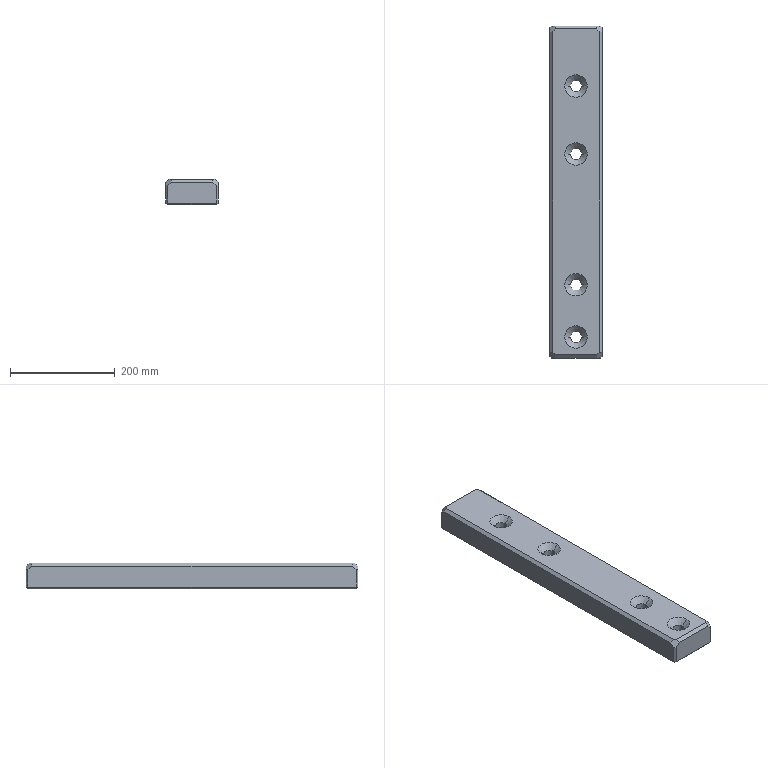Part | Creo | 1 solid | 50 faces | box 100 x 635 x 49.3 mm | volume 3002478 mm3 | plane 26 | cone 16 | cylinder 8 | commonest cylinder face diameters 21.5 x8
STEP:
#1=CARTESIAN_POINT('',(0.,0.,0.));
#2=DIRECTION('',(0.,0.,1.));
#3=DIRECTION('',(1.,0.,0.));
#4=AXIS2_PLACEMENT_3D('',#1,#2,#3);
#5=CARTESIAN_POINT('',(-246.47,-323.899,305.059));
#6=VERTEX_POINT('',#5);
#7=CARTESIAN_POINT('',(-325.328,-323.899,305.059));
#8=VERTEX_POINT('',#7);
#9=CARTESIAN_POINT('',(-246.47,-323.899,305.059));
#10=DIRECTION('',(-1.,0.,0.));
#11=VECTOR('',#10,78.858);
#12=LINE('',#9,#11);
#13=EDGE_CURVE('',#6,#8,#12,.T.);
#14=ORIENTED_EDGE('',*,*,#13,.T.);
#15=CARTESIAN_POINT('',(-330.17,-319.056,305.059));
#16=VERTEX_POINT('',#15);
#17=CARTESIAN_POINT('',(-325.328,-323.899,305.059));
#18=DIRECTION('',(-0.7071,0.7071,0.));
#19=VECTOR('',#18,6.848);
#20=LINE('',#17,#19);
#21=EDGE_CURVE('',#8,#16,#20,.T.);
#22=ORIENTED_EDGE('',*,*,#21,.T.);
#23=CARTESIAN_POINT('',(-330.17,294.801,305.059));
#24=VERTEX_POINT('',#23);
#25=CARTESIAN_POINT('',(-330.17,-319.056,305.059));
#26=DIRECTION('',(0.,1.,0.));
#27=VECTOR('',#26,613.858);
#28=LINE('',#25,#27);
#29=EDGE_CURVE('',#16,#24,#28,.T.);
#30=ORIENTED_EDGE('',*,*,#29,.T.);
#31=CARTESIAN_POINT('',(-325.328,299.644,305.059));
#32=VERTEX_POINT('',#31);
#33=CARTESIAN_POINT('',(-330.17,294.801,305.059));
#34=DIRECTION('',(0.7071,0.7071,0.));
#35=VECTOR('',#34,6.848);
#36=LINE('',#33,#35);
#37=EDGE_CURVE('',#24,#32,#36,.T.);
#38=ORIENTED_EDGE('',*,*,#37,.T.);
#39=CARTESIAN_POINT('',(-246.47,299.644,305.059));
#40=VERTEX_POINT('',#39);
#41=CARTESIAN_POINT('',(-325.328,299.644,305.059));
#42=DIRECTION('',(1.,0.,0.));
#43=VECTOR('',#42,78.858);
#44=LINE('',#41,#43);
#45=EDGE_CURVE('',#32,#40,#44,.T.);
#46=ORIENTED_EDGE('',*,*,#45,.T.);
#47=CARTESIAN_POINT('',(-241.628,294.801,305.059));
#48=VERTEX_POINT('',#47);
#49=CARTESIAN_POINT('',(-241.628,294.801,305.059));
#50=DIRECTION('',(-0.7071,0.7071,0.));
#51=VECTOR('',#50,6.848);
#52=LINE('',#49,#51);
#53=EDGE_CURVE('',#48,#40,#52,.T.);
#54=ORIENTED_EDGE('',*,*,#53,.F.);
#55=CARTESIAN_POINT('',(-241.628,-319.056,305.059));
#56=VERTEX_POINT('',#55);
#57=CARTESIAN_POINT('',(-241.628,294.801,305.059));
#58=DIRECTION('',(0.,-1.,0.));
#59=VECTOR('',#58,613.858);
#60=LINE('',#57,#59);
#61=EDGE_CURVE('',#48,#56,#60,.T.);
#62=ORIENTED_EDGE('',*,*,#61,.T.);
#63=CARTESIAN_POINT('',(-241.628,-319.056,305.059));
#64=DIRECTION('',(-0.7071,-0.7071,0.));
#65=VECTOR('',#64,6.848);
#66=LINE('',#63,#65);
#67=EDGE_CURVE('',#56,#6,#66,.T.);
#68=ORIENTED_EDGE('',*,*,#67,.T.);
#69=EDGE_LOOP('',(#14,#22,#30,#38,#46,#54,#62,#68));
#70=FACE_OUTER_BOUND('',#69,.F.);
#71=CARTESIAN_POINT('',(-264.349,190.373,305.059));
#72=VERTEX_POINT('',#71);
#73=CARTESIAN_POINT('',(-307.449,190.373,305.059));
#74=VERTEX_POINT('',#73);
#75=CARTESIAN_POINT('',(-285.899,190.373,305.059));
#76=DIRECTION('',(0.,0.,-1.));
#77=DIRECTION('',(1.,0.,0.));
#78=AXIS2_PLACEMENT_3D('',#75,#76,#77);
#79=CIRCLE('',#78,21.55);
#80=EDGE_CURVE('',#72,#74,#79,.T.);
#81=ORIENTED_EDGE('',*,*,#80,.F.);
#82=CARTESIAN_POINT('',(-285.899,190.373,305.059));
#83=DIRECTION('',(0.,0.,-1.));
#84=DIRECTION('',(-1.,0.,0.));
#85=AXIS2_PLACEMENT_3D('',#82,#83,#84);
#86=CIRCLE('',#85,21.55);
#87=EDGE_CURVE('',#74,#72,#86,.T.);
#88=ORIENTED_EDGE('',*,*,#87,.F.);
#89=EDGE_LOOP('',(#81,#88));
#90=FACE_BOUND('',#89,.F.);
#91=CARTESIAN_POINT('',(-264.349,60.373,305.059));
#92=VERTEX_POINT('',#91);
#93=CARTESIAN_POINT('',(-307.449,60.373,305.059));
#94=VERTEX_POINT('',#93);
#95=CARTESIAN_POINT('',(-285.899,60.373,305.059));
#96=DIRECTION('',(0.,0.,-1.));
#97=DIRECTION('',(1.,0.,0.));
#98=AXIS2_PLACEMENT_3D('',#95,#96,#97);
#99=CIRCLE('',#98,21.55);
#100=EDGE_CURVE('',#92,#94,#99,.T.);
#101=ORIENTED_EDGE('',*,*,#100,.F.);
#102=CARTESIAN_POINT('',(-285.899,60.373,305.059));
#103=DIRECTION('',(0.,0.,-1.));
#104=DIRECTION('',(-1.,0.,0.));
#105=AXIS2_PLACEMENT_3D('',#102,#103,#104);
#106=CIRCLE('',#105,21.55);
#107=EDGE_CURVE('',#94,#92,#106,.T.);
#108=ORIENTED_EDGE('',*,*,#107,.F.);
#109=EDGE_LOOP('',(#101,#108));
#110=FACE_BOUND('',#109,.F.);
#111=CARTESIAN_POINT('',(-264.349,-189.627,305.059));
#112=VERTEX_POINT('',#111);
#113=CARTESIAN_POINT('',(-307.449,-189.627,305.059));
#114=VERTEX_POINT('',#113);
#115=CARTESIAN_POINT('',(-285.899,-189.627,305.059));
#116=DIRECTION('',(0.,0.,-1.));
#117=DIRECTION('',(1.,0.,0.));
#118=AXIS2_PLACEMENT_3D('',#115,#116,#117);
#119=CIRCLE('',#118,21.55);
#120=EDGE_CURVE('',#112,#114,#119,.T.);
#121=ORIENTED_EDGE('',*,*,#120,.F.);
#122=CARTESIAN_POINT('',(-285.899,-189.627,305.059));
#123=DIRECTION('',(0.,0.,-1.));
#124=DIRECTION('',(-1.,0.,0.));
#125=AXIS2_PLACEMENT_3D('',#122,#123,#124);
#126=CIRCLE('',#125,21.55);
#127=EDGE_CURVE('',#114,#112,#126,.T.);
#128=ORIENTED_EDGE('',*,*,#127,.F.);
#129=EDGE_LOOP('',(#121,#128));
#130=FACE_BOUND('',#129,.F.);
#131=CARTESIAN_POINT('',(-264.349,-289.627,305.059));
#132=VERTEX_POINT('',#131);
#133=CARTESIAN_POINT('',(-307.449,-289.627,305.059));
#134=VERTEX_POINT('',#133);
#135=CARTESIAN_POINT('',(-285.899,-289.627,305.059));
#136=DIRECTION('',(0.,0.,-1.));
#137=DIRECTION('',(1.,0.,0.));
#138=AXIS2_PLACEMENT_3D('',#135,#136,#137);
#139=CIRCLE('',#138,21.55);
#140=EDGE_CURVE('',#132,#134,#139,.T.);
#141=ORIENTED_EDGE('',*,*,#140,.F.);
#142=CARTESIAN_POINT('',(-285.899,-289.627,305.059));
#143=DIRECTION('',(0.,0.,-1.));
#144=DIRECTION('',(-1.,0.,0.));
#145=AXIS2_PLACEMENT_3D('',#142,#143,#144);
#146=CIRCLE('',#145,21.55);
#147=EDGE_CURVE('',#134,#132,#146,.T.);
#148=ORIENTED_EDGE('',*,*,#147,.F.);
#149=EDGE_LOOP('',(#141,#148));
#150=FACE_BOUND('',#149,.F.);
#151=CARTESIAN_POINT('',(-335.899,305.373,305.059));
#152=DIRECTION('',(0.,0.,1.));
#153=DIRECTION('',(1.,0.,0.));
#154=AXIS2_PLACEMENT_3D('',#151,#152,#153);
#155=PLANE('',#154);
#156=ADVANCED_FACE('',(#70,#90,#110,#130,#150),#155,.T.);
#157=CARTESIAN_POINT('',(-246.47,-329.627,299.33));
#158=VERTEX_POINT('',#157);
#159=CARTESIAN_POINT('',(-246.47,-323.899,305.059));
#160=DIRECTION('',(0.,-0.7071,-0.7071));
#161=VECTOR('',#160,8.102);
#162=LINE('',#159,#161);
#163=EDGE_CURVE('',#6,#158,#162,.T.);
#164=ORIENTED_EDGE('',*,*,#163,.T.);
#165=CARTESIAN_POINT('',(-325.328,-329.627,299.33));
#166=VERTEX_POINT('',#165);
#167=CARTESIAN_POINT('',(-325.328,-329.627,299.33));
#168=DIRECTION('',(1.,0.,0.));
#169=VECTOR('',#168,78.858);
#170=LINE('',#167,#169);
#171=EDGE_CURVE('',#166,#158,#170,.T.);
#172=ORIENTED_EDGE('',*,*,#171,.F.);
#173=CARTESIAN_POINT('',(-325.328,-329.627,299.33));
#174=DIRECTION('',(0.,0.7071,0.7071));
#175=VECTOR('',#174,8.102);
#176=LINE('',#173,#175);
#177=EDGE_CURVE('',#166,#8,#176,.T.);
#178=ORIENTED_EDGE('',*,*,#177,.T.);
#179=ORIENTED_EDGE('',*,*,#13,.F.);
#180=EDGE_LOOP('',(#164,#172,#178,#179));
#181=FACE_OUTER_BOUND('',#180,.F.);
#182=CARTESIAN_POINT('',(-335.899,-329.663,299.294));
#183=DIRECTION('',(0.,0.7071,-0.7071));
#184=DIRECTION('',(0.,0.7071,0.7071));
#185=AXIS2_PLACEMENT_3D('',#182,#183,#184);
#186=PLANE('',#185);
#187=ADVANCED_FACE('',(#181),#186,.F.);
#188=ORIENTED_EDGE('',*,*,#67,.F.);
#189=CARTESIAN_POINT('',(-235.899,-319.056,299.33));
#190=VERTEX_POINT('',#189);
#191=CARTESIAN_POINT('',(-235.899,-319.056,299.33));
#192=DIRECTION('',(-0.7071,0.,0.7071));
#193=VECTOR('',#192,8.102);
#194=LINE('',#191,#193);
#195=EDGE_CURVE('',#190,#56,#194,.T.);
#196=ORIENTED_EDGE('',*,*,#195,.F.);
#197=CARTESIAN_POINT('',(-235.899,-326.127,292.259));
#198=VERTEX_POINT('',#197);
#199=CARTESIAN_POINT('',(-235.899,-319.056,299.33));
#200=DIRECTION('',(0.,-0.7071,-0.7071));
#201=VECTOR('',#200,10.);
#202=LINE('',#199,#201);
#203=EDGE_CURVE('',#190,#198,#202,.T.);
#204=ORIENTED_EDGE('',*,*,#203,.T.);
#205=CARTESIAN_POINT('',(-239.399,-329.627,292.259));
#206=VERTEX_POINT('',#205);
#207=CARTESIAN_POINT('',(-239.399,-329.627,292.259));
#208=DIRECTION('',(0.7071,0.7071,0.));
#209=VECTOR('',#208,4.95);
#210=LINE('',#207,#209);
#211=EDGE_CURVE('',#206,#198,#210,.T.);
#212=ORIENTED_EDGE('',*,*,#211,.F.);
#213=CARTESIAN_POINT('',(-239.399,-329.627,292.259));
#214=DIRECTION('',(-0.7071,0.,0.7071));
#215=VECTOR('',#214,10.);
#216=LINE('',#213,#215);
#217=EDGE_CURVE('',#206,#158,#216,.T.);
#218=ORIENTED_EDGE('',*,*,#217,.T.);
#219=ORIENTED_EDGE('',*,*,#163,.F.);
#220=EDGE_LOOP('',(#188,#196,#204,#212,#218,#219));
#221=FACE_OUTER_BOUND('',#220,.F.);
#222=CARTESIAN_POINT('',(-235.899,-326.127,292.259));
#223=DIRECTION('',(0.5774,-0.5774,0.5774));
#224=DIRECTION('',(0.7071,0.,-0.7071));
#225=AXIS2_PLACEMENT_3D('',#222,#223,#224);
#226=PLANE('',#225);
#227=ADVANCED_FACE('',(#221),#226,.T.);
#228=ORIENTED_EDGE('',*,*,#61,.F.);
#229=CARTESIAN_POINT('',(-235.899,294.801,299.33));
#230=VERTEX_POINT('',#229);
#231=CARTESIAN_POINT('',(-241.628,294.801,305.059));
#232=DIRECTION('',(0.7071,0.,-0.7071));
#233=VECTOR('',#232,8.102);
#234=LINE('',#231,#233);
#235=EDGE_CURVE('',#48,#230,#234,.T.);
#236=ORIENTED_EDGE('',*,*,#235,.T.);
#237=CARTESIAN_POINT('',(-235.899,-319.056,299.33));
#238=DIRECTION('',(0.,1.,0.));
#239=VECTOR('',#238,613.858);
#240=LINE('',#237,#239);
#241=EDGE_CURVE('',#190,#230,#240,.T.);
#242=ORIENTED_EDGE('',*,*,#241,.F.);
#243=ORIENTED_EDGE('',*,*,#195,.T.);
#244=EDGE_LOOP('',(#228,#236,#242,#243));
#245=FACE_OUTER_BOUND('',#244,.F.);
#246=CARTESIAN_POINT('',(-232.364,305.373,295.794));
#247=DIRECTION('',(0.7071,0.,0.7071));
#248=DIRECTION('',(0.7071,0.,-0.7071));
#249=AXIS2_PLACEMENT_3D('',#246,#247,#248);
#250=PLANE('',#249);
#251=ADVANCED_FACE('',(#245),#250,.T.);
#252=CARTESIAN_POINT('',(-246.47,305.373,299.33));
#253=VERTEX_POINT('',#252);
#254=CARTESIAN_POINT('',(-246.47,305.373,299.33));
#255=DIRECTION('',(0.,-0.7071,0.7071));
#256=VECTOR('',#255,8.102);
#257=LINE('',#254,#256);
#258=EDGE_CURVE('',#253,#40,#257,.T.);
#259=ORIENTED_EDGE('',*,*,#258,.F.);
#260=CARTESIAN_POINT('',(-239.399,305.373,292.259));
#261=VERTEX_POINT('',#260);
#262=CARTESIAN_POINT('',(-246.47,305.373,299.33));
#263=DIRECTION('',(0.7071,0.,-0.7071));
#264=VECTOR('',#263,10.);
#265=LINE('',#262,#264);
#266=EDGE_CURVE('',#253,#261,#265,.T.);
#267=ORIENTED_EDGE('',*,*,#266,.T.);
#268=CARTESIAN_POINT('',(-235.899,301.873,292.259));
#269=VERTEX_POINT('',#268);
#270=CARTESIAN_POINT('',(-235.899,301.873,292.259));
#271=DIRECTION('',(-0.7071,0.7071,0.));
#272=VECTOR('',#271,4.95);
#273=LINE('',#270,#272);
#274=EDGE_CURVE('',#269,#261,#273,.T.);
#275=ORIENTED_EDGE('',*,*,#274,.F.);
#276=CARTESIAN_POINT('',(-235.899,301.873,292.259));
#277=DIRECTION('',(0.,-0.7071,0.7071));
#278=VECTOR('',#277,10.);
#279=LINE('',#276,#278);
#280=EDGE_CURVE('',#269,#230,#279,.T.);
#281=ORIENTED_EDGE('',*,*,#280,.T.);
#282=ORIENTED_EDGE('',*,*,#235,.F.);
#283=ORIENTED_EDGE('',*,*,#53,.T.);
#284=EDGE_LOOP('',(#259,#267,#275,#281,#282,#283));
#285=FACE_OUTER_BOUND('',#284,.F.);
#286=CARTESIAN_POINT('',(-239.399,301.873,295.759));
#287=DIRECTION('',(0.5774,0.5774,0.5774));
#288=DIRECTION('',(0.,-0.7071,0.7071));
#289=AXIS2_PLACEMENT_3D('',#286,#287,#288);
#290=PLANE('',#289);
#291=ADVANCED_FACE('',(#285),#290,.T.);
#292=ORIENTED_EDGE('',*,*,#45,.F.);
#293=CARTESIAN_POINT('',(-325.328,305.373,299.33));
#294=VERTEX_POINT('',#293);
#295=CARTESIAN_POINT('',(-325.328,299.644,305.059));
#296=DIRECTION('',(0.,0.7071,-0.7071));
#297=VECTOR('',#296,8.102);
#298=LINE('',#295,#297);
#299=EDGE_CURVE('',#32,#294,#298,.T.);
#300=ORIENTED_EDGE('',*,*,#299,.T.);
#301=CARTESIAN_POINT('',(-246.47,305.373,299.33));
#302=DIRECTION('',(-1.,0.,0.));
#303=VECTOR('',#302,78.858);
#304=LINE('',#301,#303);
#305=EDGE_CURVE('',#253,#294,#304,.T.);
#306=ORIENTED_EDGE('',*,*,#305,.F.);
#307=ORIENTED_EDGE('',*,*,#258,.T.);
#308=EDGE_LOOP('',(#292,#300,#306,#307));
#309=FACE_OUTER_BOUND('',#308,.F.);
#310=CARTESIAN_POINT('',(-335.899,308.908,295.794));
#311=DIRECTION('',(0.,0.7071,0.7071));
#312=DIRECTION('',(0.,-0.7071,0.7071));
#313=AXIS2_PLACEMENT_3D('',#310,#311,#312);
#314=PLANE('',#313);
#315=ADVANCED_FACE('',(#309),#314,.T.);
#316=ORIENTED_EDGE('',*,*,#37,.F.);
#317=CARTESIAN_POINT('',(-335.899,294.801,299.33));
#318=VERTEX_POINT('',#317);
#319=CARTESIAN_POINT('',(-330.17,294.801,305.059));
#320=DIRECTION('',(-0.7071,0.,-0.7071));
#321=VECTOR('',#320,8.102);
#322=LINE('',#319,#321);
#323=EDGE_CURVE('',#24,#318,#322,.T.);
#324=ORIENTED_EDGE('',*,*,#323,.T.);
#325=CARTESIAN_POINT('',(-335.899,301.873,292.259));
#326=VERTEX_POINT('',#325);
#327=CARTESIAN_POINT('',(-335.899,294.801,299.33));
#328=DIRECTION('',(0.,0.7071,-0.7071));
#329=VECTOR('',#328,10.);
#330=LINE('',#327,#329);
#331=EDGE_CURVE('',#318,#326,#330,.T.);
#332=ORIENTED_EDGE('',*,*,#331,.T.);
#333=CARTESIAN_POINT('',(-332.399,305.373,292.259));
#334=VERTEX_POINT('',#333);
#335=CARTESIAN_POINT('',(-332.399,305.373,292.259));
#336=DIRECTION('',(-0.7071,-0.7071,0.));
#337=VECTOR('',#336,4.95);
#338=LINE('',#335,#337);
#339=EDGE_CURVE('',#334,#326,#338,.T.);
#340=ORIENTED_EDGE('',*,*,#339,.F.);
#341=CARTESIAN_POINT('',(-332.399,305.373,292.259));
#342=DIRECTION('',(0.7071,0.,0.7071));
#343=VECTOR('',#342,10.);
#344=LINE('',#341,#343);
#345=EDGE_CURVE('',#334,#294,#344,.T.);
#346=ORIENTED_EDGE('',*,*,#345,.T.);
#347=ORIENTED_EDGE('',*,*,#299,.F.);
#348=EDGE_LOOP('',(#316,#324,#332,#340,#346,#347));
#349=FACE_OUTER_BOUND('',#348,.F.);
#350=CARTESIAN_POINT('',(-332.399,305.373,292.259));
#351=DIRECTION('',(-0.5774,0.5774,0.5774));
#352=DIRECTION('',(0.7071,0.,0.7071));
#353=AXIS2_PLACEMENT_3D('',#350,#351,#352);
#354=PLANE('',#353);
#355=ADVANCED_FACE('',(#349),#354,.T.);
#356=CARTESIAN_POINT('',(-335.899,-319.056,299.33));
#357=VERTEX_POINT('',#356);
#358=CARTESIAN_POINT('',(-330.17,-319.056,305.059));
#359=DIRECTION('',(-0.7071,0.,-0.7071));
#360=VECTOR('',#359,8.102);
#361=LINE('',#358,#360);
#362=EDGE_CURVE('',#16,#357,#361,.T.);
#363=ORIENTED_EDGE('',*,*,#362,.T.);
#364=CARTESIAN_POINT('',(-335.899,294.801,299.33));
#365=DIRECTION('',(0.,-1.,0.));
#366=VECTOR('',#365,613.858);
#367=LINE('',#364,#366);
#368=EDGE_CURVE('',#318,#357,#367,.T.);
#369=ORIENTED_EDGE('',*,*,#368,.F.);
#370=ORIENTED_EDGE('',*,*,#323,.F.);
#371=ORIENTED_EDGE('',*,*,#29,.F.);
#372=EDGE_LOOP('',(#363,#369,#370,#371));
#373=FACE_OUTER_BOUND('',#372,.F.);
#374=CARTESIAN_POINT('',(-335.935,305.373,299.294));
#375=DIRECTION('',(0.7071,0.,-0.7071));
#376=DIRECTION('',(-0.7071,0.,-0.7071));
#377=AXIS2_PLACEMENT_3D('',#374,#375,#376);
#378=PLANE('',#377);
#379=ADVANCED_FACE('',(#373),#378,.F.);
#380=ORIENTED_EDGE('',*,*,#21,.F.);
#381=ORIENTED_EDGE('',*,*,#177,.F.);
#382=CARTESIAN_POINT('',(-332.399,-329.627,292.259));
#383=VERTEX_POINT('',#382);
#384=CARTESIAN_POINT('',(-325.328,-329.627,299.33));
#385=DIRECTION('',(-0.7071,0.,-0.7071));
#386=VECTOR('',#385,10.);
#387=LINE('',#384,#386);
#388=EDGE_CURVE('',#166,#383,#387,.T.);
#389=ORIENTED_EDGE('',*,*,#388,.T.);
#390=CARTESIAN_POINT('',(-335.899,-326.127,292.259));
#391=VERTEX_POINT('',#390);
#392=CARTESIAN_POINT('',(-335.899,-326.127,292.259));
#393=DIRECTION('',(0.7071,-0.7071,0.));
#394=VECTOR('',#393,4.95);
#395=LINE('',#392,#394);
#396=EDGE_CURVE('',#391,#383,#395,.T.);
#397=ORIENTED_EDGE('',*,*,#396,.F.);
#398=CARTESIAN_POINT('',(-335.899,-319.056,299.33));
#399=DIRECTION('',(0.,-0.7071,-0.7071));
#400=VECTOR('',#399,10.);
#401=LINE('',#398,#400);
#402=EDGE_CURVE('',#357,#391,#401,.T.);
#403=ORIENTED_EDGE('',*,*,#402,.F.);
#404=ORIENTED_EDGE('',*,*,#362,.F.);
#405=EDGE_LOOP('',(#380,#381,#389,#397,#403,#404));
#406=FACE_OUTER_BOUND('',#405,.F.);
#407=CARTESIAN_POINT('',(-335.899,-326.127,292.259));
#408=DIRECTION('',(-0.5774,-0.5774,0.5774));
#409=DIRECTION('',(0.7071,0.,0.7071));
#410=AXIS2_PLACEMENT_3D('',#407,#408,#409);
#411=PLANE('',#410);
#412=ADVANCED_FACE('',(#406),#411,.T.);
#413=CARTESIAN_POINT('',(-239.399,-329.627,259.259));
#414=VERTEX_POINT('',#413);
#415=CARTESIAN_POINT('',(-332.399,-329.627,259.259));
#416=VERTEX_POINT('',#415);
#417=CARTESIAN_POINT('',(-239.399,-329.627,259.259));
#418=DIRECTION('',(-1.,0.,0.));
#419=VECTOR('',#418,93.);
#420=LINE('',#417,#419);
#421=EDGE_CURVE('',#414,#416,#420,.T.);
#422=ORIENTED_EDGE('',*,*,#421,.T.);
#423=CARTESIAN_POINT('',(-332.399,-329.627,259.259));
#424=DIRECTION('',(0.,0.,1.));
#425=VECTOR('',#424,33.);
#426=LINE('',#423,#425);
#427=EDGE_CURVE('',#416,#383,#426,.T.);
#428=ORIENTED_EDGE('',*,*,#427,.T.);
#429=ORIENTED_EDGE('',*,*,#388,.F.);
#430=ORIENTED_EDGE('',*,*,#171,.T.);
#431=ORIENTED_EDGE('',*,*,#217,.F.);
#432=CARTESIAN_POINT('',(-239.399,-329.627,292.259));
#433=DIRECTION('',(0.,0.,-1.));
#434=VECTOR('',#433,33.);
#435=LINE('',#432,#434);
#436=EDGE_CURVE('',#206,#414,#435,.T.);
#437=ORIENTED_EDGE('',*,*,#436,.T.);
#438=EDGE_LOOP('',(#422,#428,#429,#430,#431,#437));
#439=FACE_OUTER_BOUND('',#438,.F.);
#440=CARTESIAN_POINT('',(-335.899,-329.627,290.759));
#441=DIRECTION('',(0.,-1.,0.));
#442=DIRECTION('',(1.,0.,0.));
#443=AXIS2_PLACEMENT_3D('',#440,#441,#442);
#444=PLANE('',#443);
#445=ADVANCED_FACE('',(#439),#444,.T.);
#446=CARTESIAN_POINT('',(-239.399,-326.127,255.759));
#447=VERTEX_POINT('',#446);
#448=CARTESIAN_POINT('',(-239.399,-329.627,259.259));
#449=DIRECTION('',(0.,0.7071,-0.7071));
#450=VECTOR('',#449,4.95);
#451=LINE('',#448,#450);
#452=EDGE_CURVE('',#414,#447,#451,.T.);
#453=ORIENTED_EDGE('',*,*,#452,.T.);
#454=CARTESIAN_POINT('',(-332.399,-326.127,255.759));
#455=VERTEX_POINT('',#454);
#456=CARTESIAN_POINT('',(-332.399,-326.127,255.759));
#457=DIRECTION('',(1.,0.,0.));
#458=VECTOR('',#457,93.);
#459=LINE('',#456,#458);
#460=EDGE_CURVE('',#455,#447,#459,.T.);
#461=ORIENTED_EDGE('',*,*,#460,.F.);
#462=CARTESIAN_POINT('',(-332.399,-326.127,255.759));
#463=DIRECTION('',(0.,-0.7071,0.7071));
#464=VECTOR('',#463,4.95);
#465=LINE('',#462,#464);
#466=EDGE_CURVE('',#455,#416,#465,.T.);
#467=ORIENTED_EDGE('',*,*,#466,.T.);
#468=ORIENTED_EDGE('',*,*,#421,.F.);
#469=EDGE_LOOP('',(#453,#461,#467,#468));
#470=FACE_OUTER_BOUND('',#469,.F.);
#471=CARTESIAN_POINT('',(-335.899,-329.627,259.259));
#472=DIRECTION('',(0.,-0.7071,-0.7071));
#473=DIRECTION('',(0.,0.7071,-0.7071));
#474=AXIS2_PLACEMENT_3D('',#471,#472,#473);
#475=PLANE('',#474);
#476=ADVANCED_FACE('',(#470),#475,.T.);
#477=CARTESIAN_POINT('',(-235.899,-326.127,259.259));
#478=VERTEX_POINT('',#477);
#479=CARTESIAN_POINT('',(-239.399,-326.127,255.759));
#480=DIRECTION('',(0.7071,0.,0.7071));
#481=VECTOR('',#480,4.95);
#482=LINE('',#479,#481);
#483=EDGE_CURVE('',#447,#478,#482,.T.);
#484=ORIENTED_EDGE('',*,*,#483,.F.);
#485=ORIENTED_EDGE('',*,*,#452,.F.);
#486=CARTESIAN_POINT('',(-235.899,-326.127,259.259));
#487=DIRECTION('',(-0.7071,-0.7071,0.));
#488=VECTOR('',#487,4.95);
#489=LINE('',#486,#488);
#490=EDGE_CURVE('',#478,#414,#489,.T.);
#491=ORIENTED_EDGE('',*,*,#490,.F.);
#492=EDGE_LOOP('',(#484,#485,#491));
#493=FACE_OUTER_BOUND('',#492,.F.);
#494=CARTESIAN_POINT('',(-235.899,-326.127,259.259));
#495=DIRECTION('',(0.5774,-0.5774,-0.5774));
#496=DIRECTION('',(-0.7071,0.,-0.7071));
#497=AXIS2_PLACEMENT_3D('',#494,#495,#496);
#498=PLANE('',#497);
#499=ADVANCED_FACE('',(#493),#498,.T.);
#500=ORIENTED_EDGE('',*,*,#483,.T.);
#501=CARTESIAN_POINT('',(-235.899,301.873,259.259));
#502=VERTEX_POINT('',#501);
#503=CARTESIAN_POINT('',(-235.899,301.873,259.259));
#504=DIRECTION('',(0.,-1.,0.));
#505=VECTOR('',#504,628.);
#506=LINE('',#503,#505);
#507=EDGE_CURVE('',#502,#478,#506,.T.);
#508=ORIENTED_EDGE('',*,*,#507,.F.);
#509=CARTESIAN_POINT('',(-239.399,301.873,255.759));
#510=VERTEX_POINT('',#509);
#511=CARTESIAN_POINT('',(-235.899,301.873,259.259));
#512=DIRECTION('',(-0.7071,0.,-0.7071));
#513=VECTOR('',#512,4.95);
#514=LINE('',#511,#513);
#515=EDGE_CURVE('',#502,#510,#514,.T.);
#516=ORIENTED_EDGE('',*,*,#515,.T.);
#517=CARTESIAN_POINT('',(-239.399,-326.127,255.759));
#518=DIRECTION('',(0.,1.,0.));
#519=VECTOR('',#518,628.);
#520=LINE('',#517,#519);
#521=EDGE_CURVE('',#447,#510,#520,.T.);
#522=ORIENTED_EDGE('',*,*,#521,.F.);
#523=EDGE_LOOP('',(#500,#508,#516,#522));
#524=FACE_OUTER_BOUND('',#523,.F.);
#525=CARTESIAN_POINT('',(-239.399,305.373,255.759));
#526=DIRECTION('',(-0.7071,0.,0.7071));
#527=DIRECTION('',(0.7071,0.,0.7071));
#528=AXIS2_PLACEMENT_3D('',#525,#526,#527);
#529=PLANE('',#528);
#530=ADVANCED_FACE('',(#524),#529,.F.);
#531=CARTESIAN_POINT('',(-235.899,301.873,292.259));
#532=DIRECTION('',(0.,0.,-1.));
#533=VECTOR('',#532,33.);
#534=LINE('',#531,#533);
#535=EDGE_CURVE('',#269,#502,#534,.T.);
#536=ORIENTED_EDGE('',*,*,#535,.T.);
#537=ORIENTED_EDGE('',*,*,#507,.T.);
#538=CARTESIAN_POINT('',(-235.899,-326.127,259.259));
#539=DIRECTION('',(0.,0.,1.));
#540=VECTOR('',#539,33.);
#541=LINE('',#538,#540);
#542=EDGE_CURVE('',#478,#198,#541,.T.);
#543=ORIENTED_EDGE('',*,*,#542,.T.);
#544=ORIENTED_EDGE('',*,*,#203,.F.);
#545=ORIENTED_EDGE('',*,*,#241,.T.);
#546=ORIENTED_EDGE('',*,*,#280,.F.);
#547=EDGE_LOOP('',(#536,#537,#543,#544,#545,#546));
#548=FACE_OUTER_BOUND('',#547,.F.);
#549=CARTESIAN_POINT('',(-235.899,305.373,290.759));
#550=DIRECTION('',(-1.,0.,0.));
#551=DIRECTION('',(0.,-1.,0.));
#552=AXIS2_PLACEMENT_3D('',#549,#550,#551);
#553=PLANE('',#552);
#554=ADVANCED_FACE('',(#548),#553,.F.);
#555=ORIENTED_EDGE('',*,*,#274,.T.);
#556=CARTESIAN_POINT('',(-239.399,305.373,259.259));
#557=VERTEX_POINT('',#556);
#558=CARTESIAN_POINT('',(-239.399,305.373,259.259));
#559=DIRECTION('',(0.,0.,1.));
#560=VECTOR('',#559,33.);
#561=LINE('',#558,#560);
#562=EDGE_CURVE('',#557,#261,#561,.T.);
#563=ORIENTED_EDGE('',*,*,#562,.F.);
#564=CARTESIAN_POINT('',(-239.399,305.373,259.259));
#565=DIRECTION('',(0.7071,-0.7071,0.));
#566=VECTOR('',#565,4.95);
#567=LINE('',#564,#566);
#568=EDGE_CURVE('',#557,#502,#567,.T.);
#569=ORIENTED_EDGE('',*,*,#568,.T.);
#570=ORIENTED_EDGE('',*,*,#535,.F.);
#571=EDGE_LOOP('',(#555,#563,#569,#570));
#572=FACE_OUTER_BOUND('',#571,.F.);
#573=CARTESIAN_POINT('',(-239.399,305.373,290.759));
#574=DIRECTION('',(-0.7071,-0.7071,0.));
#575=DIRECTION('',(0.7071,-0.7071,0.));
#576=AXIS2_PLACEMENT_3D('',#573,#574,#575);
#577=PLANE('',#576);
#578=ADVANCED_FACE('',(#572),#577,.F.);
#579=CARTESIAN_POINT('',(-332.399,305.373,259.259));
#580=VERTEX_POINT('',#579);
#581=CARTESIAN_POINT('',(-332.399,305.373,259.259));
#582=DIRECTION('',(1.,0.,0.));
#583=VECTOR('',#582,93.);
#584=LINE('',#581,#583);
#585=EDGE_CURVE('',#580,#557,#584,.T.);
#586=ORIENTED_EDGE('',*,*,#585,.T.);
#587=ORIENTED_EDGE('',*,*,#562,.T.);
#588=ORIENTED_EDGE('',*,*,#266,.F.);
#589=ORIENTED_EDGE('',*,*,#305,.T.);
#590=ORIENTED_EDGE('',*,*,#345,.F.);
#591=CARTESIAN_POINT('',(-332.399,305.373,292.259));
#592=DIRECTION('',(0.,0.,-1.));
#593=VECTOR('',#592,33.);
#594=LINE('',#591,#593);
#595=EDGE_CURVE('',#334,#580,#594,.T.);
#596=ORIENTED_EDGE('',*,*,#595,.T.);
#597=EDGE_LOOP('',(#586,#587,#588,#589,#590,#596));
#598=FACE_OUTER_BOUND('',#597,.F.);
#599=CARTESIAN_POINT('',(-335.899,305.373,290.759));
#600=DIRECTION('',(0.,-1.,0.));
#601=DIRECTION('',(1.,0.,0.));
#602=AXIS2_PLACEMENT_3D('',#599,#600,#601);
#603=PLANE('',#602);
#604=ADVANCED_FACE('',(#598),#603,.F.);
#605=CARTESIAN_POINT('',(-239.399,301.873,255.759));
#606=DIRECTION('',(0.,0.7071,0.7071));
#607=VECTOR('',#606,4.95);
#608=LINE('',#605,#607);
#609=EDGE_CURVE('',#510,#557,#608,.T.);
#610=ORIENTED_EDGE('',*,*,#609,.T.);
#611=ORIENTED_EDGE('',*,*,#585,.F.);
#612=CARTESIAN_POINT('',(-332.399,301.873,255.759));
#613=VERTEX_POINT('',#612);
#614=CARTESIAN_POINT('',(-332.399,305.373,259.259));
#615=DIRECTION('',(0.,-0.7071,-0.7071));
#616=VECTOR('',#615,4.95);
#617=LINE('',#614,#616);
#618=EDGE_CURVE('',#580,#613,#617,.T.);
#619=ORIENTED_EDGE('',*,*,#618,.T.);
#620=CARTESIAN_POINT('',(-239.399,301.873,255.759));
#621=DIRECTION('',(-1.,0.,0.));
#622=VECTOR('',#621,93.);
#623=LINE('',#620,#622);
#624=EDGE_CURVE('',#510,#613,#623,.T.);
#625=ORIENTED_EDGE('',*,*,#624,.F.);
#626=EDGE_LOOP('',(#610,#611,#619,#625));
#627=FACE_OUTER_BOUND('',#626,.F.);
#628=CARTESIAN_POINT('',(-335.899,301.873,255.759));
#629=DIRECTION('',(0.,-0.7071,0.7071));
#630=DIRECTION('',(0.,-0.7071,-0.7071));
#631=AXIS2_PLACEMENT_3D('',#628,#629,#630);
#632=PLANE('',#631);
#633=ADVANCED_FACE('',(#627),#632,.F.);
#634=ORIENTED_EDGE('',*,*,#568,.F.);
#635=ORIENTED_EDGE('',*,*,#609,.F.);
#636=ORIENTED_EDGE('',*,*,#515,.F.);
#637=EDGE_LOOP('',(#634,#635,#636));
#638=FACE_OUTER_BOUND('',#637,.F.);
#639=CARTESIAN_POINT('',(-239.399,301.873,255.759));
#640=DIRECTION('',(0.5774,0.5774,-0.5774));
#641=DIRECTION('',(0.,0.7071,0.7071));
#642=AXIS2_PLACEMENT_3D('',#639,#640,#641);
#643=PLANE('',#642);
#644=ADVANCED_FACE('',(#638),#643,.T.);
#645=ORIENTED_EDGE('',*,*,#618,.F.);
#646=CARTESIAN_POINT('',(-335.899,301.873,259.259));
#647=VERTEX_POINT('',#646);
#648=CARTESIAN_POINT('',(-335.899,301.873,259.259));
#649=DIRECTION('',(0.7071,0.7071,0.));
#650=VECTOR('',#649,4.95);
#651=LINE('',#648,#650);
#652=EDGE_CURVE('',#647,#580,#651,.T.);
#653=ORIENTED_EDGE('',*,*,#652,.F.);
#654=CARTESIAN_POINT('',(-335.899,301.873,259.259));
#655=DIRECTION('',(0.7071,0.,-0.7071));
#656=VECTOR('',#655,4.95);
#657=LINE('',#654,#656);
#658=EDGE_CURVE('',#647,#613,#657,.T.);
#659=ORIENTED_EDGE('',*,*,#658,.T.);
#660=EDGE_LOOP('',(#645,#653,#659));
#661=FACE_OUTER_BOUND('',#660,.F.);
#662=CARTESIAN_POINT('',(-335.899,301.873,259.259));
#663=DIRECTION('',(-0.5774,0.5774,-0.5774));
#664=DIRECTION('',(-0.7071,0.,0.7071));
#665=AXIS2_PLACEMENT_3D('',#662,#663,#664);
#666=PLANE('',#665);
#667=ADVANCED_FACE('',(#661),#666,.T.);
#668=ORIENTED_EDGE('',*,*,#339,.T.);
#669=CARTESIAN_POINT('',(-335.899,301.873,259.259));
#670=DIRECTION('',(0.,0.,1.));
#671=VECTOR('',#670,33.);
#672=LINE('',#669,#671);
#673=EDGE_CURVE('',#647,#326,#672,.T.);
#674=ORIENTED_EDGE('',*,*,#673,.F.);
#675=ORIENTED_EDGE('',*,*,#652,.T.);
#676=ORIENTED_EDGE('',*,*,#595,.F.);
#677=EDGE_LOOP('',(#668,#674,#675,#676));
#678=FACE_OUTER_BOUND('',#677,.F.);
#679=CARTESIAN_POINT('',(-335.899,301.873,290.759));
#680=DIRECTION('',(-0.7071,0.7071,0.));
#681=DIRECTION('',(-0.7071,-0.7071,0.));
#682=AXIS2_PLACEMENT_3D('',#679,#680,#681);
#683=PLANE('',#682);
#684=ADVANCED_FACE('',(#678),#683,.T.);
#685=ORIENTED_EDGE('',*,*,#368,.T.);
#686=ORIENTED_EDGE('',*,*,#402,.T.);
#687=CARTESIAN_POINT('',(-335.899,-326.127,259.259));
#688=VERTEX_POINT('',#687);
#689=CARTESIAN_POINT('',(-335.899,-326.127,292.259));
#690=DIRECTION('',(0.,0.,-1.));
#691=VECTOR('',#690,33.);
#692=LINE('',#689,#691);
#693=EDGE_CURVE('',#391,#688,#692,.T.);
#694=ORIENTED_EDGE('',*,*,#693,.T.);
#695=CARTESIAN_POINT('',(-335.899,-326.127,259.259));
#696=DIRECTION('',(0.,1.,0.));
#697=VECTOR('',#696,628.);
#698=LINE('',#695,#697);
#699=EDGE_CURVE('',#688,#647,#698,.T.);
#700=ORIENTED_EDGE('',*,*,#699,.T.);
#701=ORIENTED_EDGE('',*,*,#673,.T.);
#702=ORIENTED_EDGE('',*,*,#331,.F.);
#703=EDGE_LOOP('',(#685,#686,#694,#700,#701,#702));
#704=FACE_OUTER_BOUND('',#703,.F.);
#705=CARTESIAN_POINT('',(-335.899,305.373,290.759));
#706=DIRECTION('',(-1.,0.,0.));
#707=DIRECTION('',(0.,-1.,0.));
#708=AXIS2_PLACEMENT_3D('',#705,#706,#707);
#709=PLANE('',#708);
#710=ADVANCED_FACE('',(#704),#709,.T.);
#711=CARTESIAN_POINT('',(-332.399,-329.627,259.259));
#712=DIRECTION('',(-0.7071,0.7071,0.));
#713=VECTOR('',#712,4.95);
#714=LINE('',#711,#713);
#715=EDGE_CURVE('',#416,#688,#714,.T.);
#716=ORIENTED_EDGE('',*,*,#715,.T.);
#717=ORIENTED_EDGE('',*,*,#693,.F.);
#718=ORIENTED_EDGE('',*,*,#396,.T.);
#719=ORIENTED_EDGE('',*,*,#427,.F.);
#720=EDGE_LOOP('',(#716,#717,#718,#719));
#721=FACE_OUTER_BOUND('',#720,.F.);
#722=CARTESIAN_POINT('',(-332.399,-329.627,290.759));
#723=DIRECTION('',(0.7071,0.7071,0.));
#724=DIRECTION('',(-0.7071,0.7071,0.));
#725=AXIS2_PLACEMENT_3D('',#722,#723,#724);
#726=PLANE('',#725);
#727=ADVANCED_FACE('',(#721),#726,.F.);
#728=ORIENTED_EDGE('',*,*,#466,.F.);
#729=CARTESIAN_POINT('',(-335.899,-326.127,259.259));
#730=DIRECTION('',(0.7071,0.,-0.7071));
#731=VECTOR('',#730,4.95);
#732=LINE('',#729,#731);
#733=EDGE_CURVE('',#688,#455,#732,.T.);
#734=ORIENTED_EDGE('',*,*,#733,.F.);
#735=ORIENTED_EDGE('',*,*,#715,.F.);
#736=EDGE_LOOP('',(#728,#734,#735));
#737=FACE_OUTER_BOUND('',#736,.F.);
#738=CARTESIAN_POINT('',(-335.899,-326.127,259.259));
#739=DIRECTION('',(-0.5774,-0.5774,-0.5774));
#740=DIRECTION('',(-0.7071,0.,0.7071));
#741=AXIS2_PLACEMENT_3D('',#738,#739,#740);
#742=PLANE('',#741);
#743=ADVANCED_FACE('',(#737),#742,.T.);
#744=ORIENTED_EDGE('',*,*,#733,.T.);
#745=CARTESIAN_POINT('',(-332.399,301.873,255.759));
#746=DIRECTION('',(0.,-1.,0.));
#747=VECTOR('',#746,628.);
#748=LINE('',#745,#747);
#749=EDGE_CURVE('',#613,#455,#748,.T.);
#750=ORIENTED_EDGE('',*,*,#749,.F.);
#751=ORIENTED_EDGE('',*,*,#658,.F.);
#752=ORIENTED_EDGE('',*,*,#699,.F.);
#753=EDGE_LOOP('',(#744,#750,#751,#752));
#754=FACE_OUTER_BOUND('',#753,.F.);
#755=CARTESIAN_POINT('',(-335.899,305.373,259.259));
#756=DIRECTION('',(-0.7071,0.,-0.7071));
#757=DIRECTION('',(-0.7071,0.,0.7071));
#758=AXIS2_PLACEMENT_3D('',#755,#756,#757);
#759=PLANE('',#758);
#760=ADVANCED_FACE('',(#754),#759,.T.);
#761=ORIENTED_EDGE('',*,*,#460,.T.);
#762=ORIENTED_EDGE('',*,*,#521,.T.);
#763=ORIENTED_EDGE('',*,*,#624,.T.);
#764=ORIENTED_EDGE('',*,*,#749,.T.);
#765=EDGE_LOOP('',(#761,#762,#763,#764));
#766=FACE_OUTER_BOUND('',#765,.F.);
#767=CARTESIAN_POINT('',(-273.649,-189.627,255.759));
#768=VERTEX_POINT('',#767);
#769=CARTESIAN_POINT('',(-298.149,-189.627,255.759));
#770=VERTEX_POINT('',#769);
#771=CARTESIAN_POINT('',(-285.899,-189.627,255.759));
#772=DIRECTION('',(0.,0.,1.));
#773=DIRECTION('',(1.,0.,0.));
#774=AXIS2_PLACEMENT_3D('',#771,#772,#773);
#775=CIRCLE('',#774,12.25);
#776=EDGE_CURVE('',#768,#770,#775,.T.);
#777=ORIENTED_EDGE('',*,*,#776,.F.);
#778=CARTESIAN_POINT('',(-285.899,-189.627,255.759));
#779=DIRECTION('',(0.,0.,1.));
#780=DIRECTION('',(-1.,0.,0.));
#781=AXIS2_PLACEMENT_3D('',#778,#779,#780);
#782=CIRCLE('',#781,12.25);
#783=EDGE_CURVE('',#770,#768,#782,.T.);
#784=ORIENTED_EDGE('',*,*,#783,.F.);
#785=EDGE_LOOP('',(#777,#784));
#786=FACE_BOUND('',#785,.F.);
#787=CARTESIAN_POINT('',(-273.649,60.373,255.759));
#788=VERTEX_POINT('',#787);
#789=CARTESIAN_POINT('',(-298.149,60.373,255.759));
#790=VERTEX_POINT('',#789);
#791=CARTESIAN_POINT('',(-285.899,60.373,255.759));
#792=DIRECTION('',(0.,0.,1.));
#793=DIRECTION('',(1.,0.,0.));
#794=AXIS2_PLACEMENT_3D('',#791,#792,#793);
#795=CIRCLE('',#794,12.25);
#796=EDGE_CURVE('',#788,#790,#795,.T.);
#797=ORIENTED_EDGE('',*,*,#796,.F.);
#798=CARTESIAN_POINT('',(-285.899,60.373,255.759));
#799=DIRECTION('',(0.,0.,1.));
#800=DIRECTION('',(-1.,0.,0.));
#801=AXIS2_PLACEMENT_3D('',#798,#799,#800);
#802=CIRCLE('',#801,12.25);
#803=EDGE_CURVE('',#790,#788,#802,.T.);
#804=ORIENTED_EDGE('',*,*,#803,.F.);
#805=EDGE_LOOP('',(#797,#804));
#806=FACE_BOUND('',#805,.F.);
#807=CARTESIAN_POINT('',(-273.649,190.373,255.759));
#808=VERTEX_POINT('',#807);
#809=CARTESIAN_POINT('',(-298.149,190.373,255.759));
#810=VERTEX_POINT('',#809);
#811=CARTESIAN_POINT('',(-285.899,190.373,255.759));
#812=DIRECTION('',(0.,0.,1.));
#813=DIRECTION('',(1.,0.,0.));
#814=AXIS2_PLACEMENT_3D('',#811,#812,#813);
#815=CIRCLE('',#814,12.25);
#816=EDGE_CURVE('',#808,#810,#815,.T.);
#817=ORIENTED_EDGE('',*,*,#816,.F.);
#818=CARTESIAN_POINT('',(-285.899,190.373,255.759));
#819=DIRECTION('',(0.,0.,1.));
#820=DIRECTION('',(-1.,0.,0.));
#821=AXIS2_PLACEMENT_3D('',#818,#819,#820);
#822=CIRCLE('',#821,12.25);
#823=EDGE_CURVE('',#810,#808,#822,.T.);
#824=ORIENTED_EDGE('',*,*,#823,.F.);
#825=EDGE_LOOP('',(#817,#824));
#826=FACE_BOUND('',#825,.F.);
#827=CARTESIAN_POINT('',(-273.649,-289.627,255.759));
#828=VERTEX_POINT('',#827);
#829=CARTESIAN_POINT('',(-298.149,-289.627,255.759));
#830=VERTEX_POINT('',#829);
#831=CARTESIAN_POINT('',(-285.899,-289.627,255.759));
#832=DIRECTION('',(0.,0.,1.));
#833=DIRECTION('',(1.,0.,0.));
#834=AXIS2_PLACEMENT_3D('',#831,#832,#833);
#835=CIRCLE('',#834,12.25);
#836=EDGE_CURVE('',#828,#830,#835,.T.);
#837=ORIENTED_EDGE('',*,*,#836,.F.);
#838=CARTESIAN_POINT('',(-285.899,-289.627,255.759));
#839=DIRECTION('',(0.,0.,1.));
#840=DIRECTION('',(-1.,0.,0.));
#841=AXIS2_PLACEMENT_3D('',#838,#839,#840);
#842=CIRCLE('',#841,12.25);
#843=EDGE_CURVE('',#830,#828,#842,.T.);
#844=ORIENTED_EDGE('',*,*,#843,.F.);
#845=EDGE_LOOP('',(#837,#844));
#846=FACE_BOUND('',#845,.F.);
#847=CARTESIAN_POINT('',(-335.899,305.373,255.759));
#848=DIRECTION('',(0.,0.,1.));
#849=DIRECTION('',(1.,0.,0.));
#850=AXIS2_PLACEMENT_3D('',#847,#848,#849);
#851=PLANE('',#850);
#852=ADVANCED_FACE('',(#766,#786,#806,#826,#846),#851,.F.);
#853=ORIENTED_EDGE('',*,*,#836,.T.);
#854=CARTESIAN_POINT('',(-296.649,-289.627,257.259));
#855=VERTEX_POINT('',#854);
#856=CARTESIAN_POINT('',(-296.649,-289.627,257.259));
#857=DIRECTION('',(-0.7071,0.,-0.7071));
#858=VECTOR('',#857,2.121);
#859=LINE('',#856,#858);
#860=EDGE_CURVE('',#855,#830,#859,.T.);
#861=ORIENTED_EDGE('',*,*,#860,.F.);
#862=CARTESIAN_POINT('',(-275.149,-289.627,257.259));
#863=VERTEX_POINT('',#862);
#864=CARTESIAN_POINT('',(-285.899,-289.627,257.259));
#865=DIRECTION('',(0.,0.,1.));
#866=DIRECTION('',(1.,0.,0.));
#867=AXIS2_PLACEMENT_3D('',#864,#865,#866);
#868=CIRCLE('',#867,10.75);
#869=EDGE_CURVE('',#863,#855,#868,.T.);
#870=ORIENTED_EDGE('',*,*,#869,.F.);
#871=CARTESIAN_POINT('',(-275.149,-289.627,257.259));
#872=DIRECTION('',(0.7071,0.,-0.7071));
#873=VECTOR('',#872,2.121);
#874=LINE('',#871,#873);
#875=EDGE_CURVE('',#863,#828,#874,.T.);
#876=ORIENTED_EDGE('',*,*,#875,.T.);
#877=EDGE_LOOP('',(#853,#861,#870,#876));
#878=FACE_OUTER_BOUND('',#877,.F.);
#879=CARTESIAN_POINT('',(-285.899,-289.627,256.509));
#880=DIRECTION('',(0.,0.,-1.));
#881=DIRECTION('',(-1.,0.,0.));
#882=AXIS2_PLACEMENT_3D('',#879,#880,#881);
#883=CONICAL_SURFACE('',#882,11.5,45.);
#884=ADVANCED_FACE('',(#878),#883,.F.);
#885=ORIENTED_EDGE('',*,*,#843,.T.);
#886=ORIENTED_EDGE('',*,*,#875,.F.);
#887=CARTESIAN_POINT('',(-285.899,-289.627,257.259));
#888=DIRECTION('',(0.,0.,1.));
#889=DIRECTION('',(-1.,0.,0.));
#890=AXIS2_PLACEMENT_3D('',#887,#888,#889);
#891=CIRCLE('',#890,10.75);
#892=EDGE_CURVE('',#855,#863,#891,.T.);
#893=ORIENTED_EDGE('',*,*,#892,.F.);
#894=ORIENTED_EDGE('',*,*,#860,.T.);
#895=EDGE_LOOP('',(#885,#886,#893,#894));
#896=FACE_OUTER_BOUND('',#895,.F.);
#897=CARTESIAN_POINT('',(-285.899,-289.627,256.509));
#898=DIRECTION('',(0.,0.,-1.));
#899=DIRECTION('',(-1.,0.,0.));
#900=AXIS2_PLACEMENT_3D('',#897,#898,#899);
#901=CONICAL_SURFACE('',#900,11.5,45.);
#902=ADVANCED_FACE('',(#896),#901,.F.);
#903=CARTESIAN_POINT('',(-275.149,-289.627,294.259));
#904=VERTEX_POINT('',#903);
#905=CARTESIAN_POINT('',(-296.649,-289.627,294.259));
#906=VERTEX_POINT('',#905);
#907=CARTESIAN_POINT('',(-285.899,-289.627,294.259));
#908=DIRECTION('',(0.,0.,-1.));
#909=DIRECTION('',(1.,0.,0.));
#910=AXIS2_PLACEMENT_3D('',#907,#908,#909);
#911=CIRCLE('',#910,10.75);
#912=EDGE_CURVE('',#904,#906,#911,.T.);
#913=ORIENTED_EDGE('',*,*,#912,.T.);
#914=CARTESIAN_POINT('',(-296.649,-289.627,294.259));
#915=DIRECTION('',(0.,0.,-1.));
#916=VECTOR('',#915,37.);
#917=LINE('',#914,#916);
#918=EDGE_CURVE('',#906,#855,#917,.T.);
#919=ORIENTED_EDGE('',*,*,#918,.T.);
#920=ORIENTED_EDGE('',*,*,#892,.T.);
#921=CARTESIAN_POINT('',(-275.149,-289.627,294.259));
#922=DIRECTION('',(0.,0.,-1.));
#923=VECTOR('',#922,37.);
#924=LINE('',#921,#923);
#925=EDGE_CURVE('',#904,#863,#924,.T.);
#926=ORIENTED_EDGE('',*,*,#925,.F.);
#927=EDGE_LOOP('',(#913,#919,#920,#926));
#928=FACE_OUTER_BOUND('',#927,.F.);
#929=CARTESIAN_POINT('',(-285.899,-289.627,344.759));
#930=DIRECTION('',(0.,0.,-1.));
#931=DIRECTION('',(-1.,0.,0.));
#932=AXIS2_PLACEMENT_3D('',#929,#930,#931);
#933=CYLINDRICAL_SURFACE('',#932,10.75);
#934=ADVANCED_FACE('',(#928),#933,.F.);
#935=ORIENTED_EDGE('',*,*,#140,.T.);
#936=CARTESIAN_POINT('',(-296.649,-289.627,294.259));
#937=DIRECTION('',(-0.7071,0.,0.7071));
#938=VECTOR('',#937,15.274);
#939=LINE('',#936,#938);
#940=EDGE_CURVE('',#906,#134,#939,.T.);
#941=ORIENTED_EDGE('',*,*,#940,.F.);
#942=ORIENTED_EDGE('',*,*,#912,.F.);
#943=CARTESIAN_POINT('',(-275.149,-289.627,294.259));
#944=DIRECTION('',(0.7071,0.,0.7071));
#945=VECTOR('',#944,15.274);
#946=LINE('',#943,#945);
#947=EDGE_CURVE('',#904,#132,#946,.T.);
#948=ORIENTED_EDGE('',*,*,#947,.T.);
#949=EDGE_LOOP('',(#935,#941,#942,#948));
#950=FACE_OUTER_BOUND('',#949,.F.);
#951=CARTESIAN_POINT('',(-285.899,-289.627,299.659));
#952=DIRECTION('',(0.,0.,1.));
#953=DIRECTION('',(1.,0.,0.));
#954=AXIS2_PLACEMENT_3D('',#951,#952,#953);
#955=CONICAL_SURFACE('',#954,16.15,45.);
#956=ADVANCED_FACE('',(#950),#955,.F.);
#957=ORIENTED_EDGE('',*,*,#147,.T.);
#958=ORIENTED_EDGE('',*,*,#947,.F.);
#959=CARTESIAN_POINT('',(-285.899,-289.627,294.259));
#960=DIRECTION('',(0.,0.,-1.));
#961=DIRECTION('',(-1.,0.,0.));
#962=AXIS2_PLACEMENT_3D('',#959,#960,#961);
#963=CIRCLE('',#962,10.75);
#964=EDGE_CURVE('',#906,#904,#963,.T.);
#965=ORIENTED_EDGE('',*,*,#964,.F.);
#966=ORIENTED_EDGE('',*,*,#940,.T.);
#967=EDGE_LOOP('',(#957,#958,#965,#966));
#968=FACE_OUTER_BOUND('',#967,.F.);
#969=CARTESIAN_POINT('',(-285.899,-289.627,299.659));
#970=DIRECTION('',(0.,0.,1.));
#971=DIRECTION('',(1.,0.,0.));
#972=AXIS2_PLACEMENT_3D('',#969,#970,#971);
#973=CONICAL_SURFACE('',#972,16.15,45.);
#974=ADVANCED_FACE('',(#968),#973,.F.);
#975=ORIENTED_EDGE('',*,*,#964,.T.);
#976=ORIENTED_EDGE('',*,*,#925,.T.);
#977=ORIENTED_EDGE('',*,*,#869,.T.);
#978=ORIENTED_EDGE('',*,*,#918,.F.);
#979=EDGE_LOOP('',(#975,#976,#977,#978));
#980=FACE_OUTER_BOUND('',#979,.F.);
#981=CARTESIAN_POINT('',(-285.899,-289.627,344.759));
#982=DIRECTION('',(0.,0.,-1.));
#983=DIRECTION('',(-1.,0.,0.));
#984=AXIS2_PLACEMENT_3D('',#981,#982,#983);
#985=CYLINDRICAL_SURFACE('',#984,10.75);
#986=ADVANCED_FACE('',(#980),#985,.F.);
#987=ORIENTED_EDGE('',*,*,#776,.T.);
#988=CARTESIAN_POINT('',(-296.649,-189.627,257.259));
#989=VERTEX_POINT('',#988);
#990=CARTESIAN_POINT('',(-296.649,-189.627,257.259));
#991=DIRECTION('',(-0.7071,0.,-0.7071));
#992=VECTOR('',#991,2.121);
#993=LINE('',#990,#992);
#994=EDGE_CURVE('',#989,#770,#993,.T.);
#995=ORIENTED_EDGE('',*,*,#994,.F.);
#996=CARTESIAN_POINT('',(-275.149,-189.627,257.259));
#997=VERTEX_POINT('',#996);
#998=CARTESIAN_POINT('',(-285.899,-189.627,257.259));
#999=DIRECTION('',(0.,0.,1.));
#1000=DIRECTION('',(1.,0.,0.));
#1001=AXIS2_PLACEMENT_3D('',#998,#999,#1000);
#1002=CIRCLE('',#1001,10.75);
#1003=EDGE_CURVE('',#997,#989,#1002,.T.);
#1004=ORIENTED_EDGE('',*,*,#1003,.F.);
#1005=CARTESIAN_POINT('',(-275.149,-189.627,257.259));
#1006=DIRECTION('',(0.7071,0.,-0.7071));
#1007=VECTOR('',#1006,2.121);
#1008=LINE('',#1005,#1007);
#1009=EDGE_CURVE('',#997,#768,#1008,.T.);
#1010=ORIENTED_EDGE('',*,*,#1009,.T.);
#1011=EDGE_LOOP('',(#987,#995,#1004,#1010));
#1012=FACE_OUTER_BOUND('',#1011,.F.);
#1013=CARTESIAN_POINT('',(-285.899,-189.627,256.509));
#1014=DIRECTION('',(0.,0.,-1.));
#1015=DIRECTION('',(-1.,0.,0.));
#1016=AXIS2_PLACEMENT_3D('',#1013,#1014,#1015);
#1017=CONICAL_SURFACE('',#1016,11.5,45.);
#1018=ADVANCED_FACE('',(#1012),#1017,.F.);
#1019=ORIENTED_EDGE('',*,*,#783,.T.);
#1020=ORIENTED_EDGE('',*,*,#1009,.F.);
#1021=CARTESIAN_POINT('',(-285.899,-189.627,257.259));
#1022=DIRECTION('',(0.,0.,1.));
#1023=DIRECTION('',(-1.,0.,0.));
#1024=AXIS2_PLACEMENT_3D('',#1021,#1022,#1023);
#1025=CIRCLE('',#1024,10.75);
#1026=EDGE_CURVE('',#989,#997,#1025,.T.);
#1027=ORIENTED_EDGE('',*,*,#1026,.F.);
#1028=ORIENTED_EDGE('',*,*,#994,.T.);
#1029=EDGE_LOOP('',(#1019,#1020,#1027,#1028));
#1030=FACE_OUTER_BOUND('',#1029,.F.);
#1031=CARTESIAN_POINT('',(-285.899,-189.627,256.509));
#1032=DIRECTION('',(0.,0.,-1.));
#1033=DIRECTION('',(-1.,0.,0.));
#1034=AXIS2_PLACEMENT_3D('',#1031,#1032,#1033);
#1035=CONICAL_SURFACE('',#1034,11.5,45.);
#1036=ADVANCED_FACE('',(#1030),#1035,.F.);
#1037=CARTESIAN_POINT('',(-275.149,-189.627,294.259));
#1038=VERTEX_POINT('',#1037);
#1039=CARTESIAN_POINT('',(-296.649,-189.627,294.259));
#1040=VERTEX_POINT('',#1039);
#1041=CARTESIAN_POINT('',(-285.899,-189.627,294.259));
#1042=DIRECTION('',(0.,0.,-1.));
#1043=DIRECTION('',(1.,0.,0.));
#1044=AXIS2_PLACEMENT_3D('',#1041,#1042,#1043);
#1045=CIRCLE('',#1044,10.75);
#1046=EDGE_CURVE('',#1038,#1040,#1045,.T.);
#1047=ORIENTED_EDGE('',*,*,#1046,.T.);
#1048=CARTESIAN_POINT('',(-296.649,-189.627,294.259));
#1049=DIRECTION('',(0.,0.,-1.));
#1050=VECTOR('',#1049,37.);
#1051=LINE('',#1048,#1050);
#1052=EDGE_CURVE('',#1040,#989,#1051,.T.);
#1053=ORIENTED_EDGE('',*,*,#1052,.T.);
#1054=ORIENTED_EDGE('',*,*,#1026,.T.);
#1055=CARTESIAN_POINT('',(-275.149,-189.627,294.259));
#1056=DIRECTION('',(0.,0.,-1.));
#1057=VECTOR('',#1056,37.);
#1058=LINE('',#1055,#1057);
#1059=EDGE_CURVE('',#1038,#997,#1058,.T.);
#1060=ORIENTED_EDGE('',*,*,#1059,.F.);
#1061=EDGE_LOOP('',(#1047,#1053,#1054,#1060));
#1062=FACE_OUTER_BOUND('',#1061,.F.);
#1063=CARTESIAN_POINT('',(-285.899,-189.627,344.759));
#1064=DIRECTION('',(0.,0.,-1.));
#1065=DIRECTION('',(-1.,0.,0.));
#1066=AXIS2_PLACEMENT_3D('',#1063,#1064,#1065);
#1067=CYLINDRICAL_SURFACE('',#1066,10.75);
#1068=ADVANCED_FACE('',(#1062),#1067,.F.);
#1069=ORIENTED_EDGE('',*,*,#120,.T.);
#1070=CARTESIAN_POINT('',(-296.649,-189.627,294.259));
#1071=DIRECTION('',(-0.7071,0.,0.7071));
#1072=VECTOR('',#1071,15.274);
#1073=LINE('',#1070,#1072);
#1074=EDGE_CURVE('',#1040,#114,#1073,.T.);
#1075=ORIENTED_EDGE('',*,*,#1074,.F.);
#1076=ORIENTED_EDGE('',*,*,#1046,.F.);
#1077=CARTESIAN_POINT('',(-275.149,-189.627,294.259));
#1078=DIRECTION('',(0.7071,0.,0.7071));
#1079=VECTOR('',#1078,15.274);
#1080=LINE('',#1077,#1079);
#1081=EDGE_CURVE('',#1038,#112,#1080,.T.);
#1082=ORIENTED_EDGE('',*,*,#1081,.T.);
#1083=EDGE_LOOP('',(#1069,#1075,#1076,#1082));
#1084=FACE_OUTER_BOUND('',#1083,.F.);
#1085=CARTESIAN_POINT('',(-285.899,-189.627,299.659));
#1086=DIRECTION('',(0.,0.,1.));
#1087=DIRECTION('',(1.,0.,0.));
#1088=AXIS2_PLACEMENT_3D('',#1085,#1086,#1087);
#1089=CONICAL_SURFACE('',#1088,16.15,45.);
#1090=ADVANCED_FACE('',(#1084),#1089,.F.);
#1091=ORIENTED_EDGE('',*,*,#127,.T.);
#1092=ORIENTED_EDGE('',*,*,#1081,.F.);
#1093=CARTESIAN_POINT('',(-285.899,-189.627,294.259));
#1094=DIRECTION('',(0.,0.,-1.));
#1095=DIRECTION('',(-1.,0.,0.));
#1096=AXIS2_PLACEMENT_3D('',#1093,#1094,#1095);
#1097=CIRCLE('',#1096,10.75);
#1098=EDGE_CURVE('',#1040,#1038,#1097,.T.);
#1099=ORIENTED_EDGE('',*,*,#1098,.F.);
#1100=ORIENTED_EDGE('',*,*,#1074,.T.);
#1101=EDGE_LOOP('',(#1091,#1092,#1099,#1100));
#1102=FACE_OUTER_BOUND('',#1101,.F.);
#1103=CARTESIAN_POINT('',(-285.899,-189.627,299.659));
#1104=DIRECTION('',(0.,0.,1.));
#1105=DIRECTION('',(1.,0.,0.));
#1106=AXIS2_PLACEMENT_3D('',#1103,#1104,#1105);
#1107=CONICAL_SURFACE('',#1106,16.15,45.);
#1108=ADVANCED_FACE('',(#1102),#1107,.F.);
#1109=ORIENTED_EDGE('',*,*,#1098,.T.);
#1110=ORIENTED_EDGE('',*,*,#1059,.T.);
#1111=ORIENTED_EDGE('',*,*,#1003,.T.);
#1112=ORIENTED_EDGE('',*,*,#1052,.F.);
#1113=EDGE_LOOP('',(#1109,#1110,#1111,#1112));
#1114=FACE_OUTER_BOUND('',#1113,.F.);
#1115=CARTESIAN_POINT('',(-285.899,-189.627,344.759));
#1116=DIRECTION('',(0.,0.,-1.));
#1117=DIRECTION('',(-1.,0.,0.));
#1118=AXIS2_PLACEMENT_3D('',#1115,#1116,#1117);
#1119=CYLINDRICAL_SURFACE('',#1118,10.75);
#1120=ADVANCED_FACE('',(#1114),#1119,.F.);
#1121=ORIENTED_EDGE('',*,*,#796,.T.);
#1122=CARTESIAN_POINT('',(-296.649,60.373,257.259));
#1123=VERTEX_POINT('',#1122);
#1124=CARTESIAN_POINT('',(-296.649,60.373,257.259));
#1125=DIRECTION('',(-0.7071,0.,-0.7071));
#1126=VECTOR('',#1125,2.121);
#1127=LINE('',#1124,#1126);
#1128=EDGE_CURVE('',#1123,#790,#1127,.T.);
#1129=ORIENTED_EDGE('',*,*,#1128,.F.);
#1130=CARTESIAN_POINT('',(-275.149,60.373,257.259));
#1131=VERTEX_POINT('',#1130);
#1132=CARTESIAN_POINT('',(-285.899,60.373,257.259));
#1133=DIRECTION('',(0.,0.,1.));
#1134=DIRECTION('',(1.,0.,0.));
#1135=AXIS2_PLACEMENT_3D('',#1132,#1133,#1134);
#1136=CIRCLE('',#1135,10.75);
#1137=EDGE_CURVE('',#1131,#1123,#1136,.T.);
#1138=ORIENTED_EDGE('',*,*,#1137,.F.);
#1139=CARTESIAN_POINT('',(-275.149,60.373,257.259));
#1140=DIRECTION('',(0.7071,0.,-0.7071));
#1141=VECTOR('',#1140,2.121);
#1142=LINE('',#1139,#1141);
#1143=EDGE_CURVE('',#1131,#788,#1142,.T.);
#1144=ORIENTED_EDGE('',*,*,#1143,.T.);
#1145=EDGE_LOOP('',(#1121,#1129,#1138,#1144));
#1146=FACE_OUTER_BOUND('',#1145,.F.);
#1147=CARTESIAN_POINT('',(-285.899,60.373,256.509));
#1148=DIRECTION('',(0.,0.,-1.));
#1149=DIRECTION('',(-1.,0.,0.));
#1150=AXIS2_PLACEMENT_3D('',#1147,#1148,#1149);
#1151=CONICAL_SURFACE('',#1150,11.5,45.);
#1152=ADVANCED_FACE('',(#1146),#1151,.F.);
#1153=ORIENTED_EDGE('',*,*,#803,.T.);
#1154=ORIENTED_EDGE('',*,*,#1143,.F.);
#1155=CARTESIAN_POINT('',(-285.899,60.373,257.259));
#1156=DIRECTION('',(0.,0.,1.));
#1157=DIRECTION('',(-1.,0.,0.));
#1158=AXIS2_PLACEMENT_3D('',#1155,#1156,#1157);
#1159=CIRCLE('',#1158,10.75);
#1160=EDGE_CURVE('',#1123,#1131,#1159,.T.);
#1161=ORIENTED_EDGE('',*,*,#1160,.F.);
#1162=ORIENTED_EDGE('',*,*,#1128,.T.);
#1163=EDGE_LOOP('',(#1153,#1154,#1161,#1162));
#1164=FACE_OUTER_BOUND('',#1163,.F.);
#1165=CARTESIAN_POINT('',(-285.899,60.373,256.509));
#1166=DIRECTION('',(0.,0.,-1.));
#1167=DIRECTION('',(-1.,0.,0.));
#1168=AXIS2_PLACEMENT_3D('',#1165,#1166,#1167);
#1169=CONICAL_SURFACE('',#1168,11.5,45.);
#1170=ADVANCED_FACE('',(#1164),#1169,.F.);
#1171=CARTESIAN_POINT('',(-275.149,60.373,294.259));
#1172=VERTEX_POINT('',#1171);
#1173=CARTESIAN_POINT('',(-296.649,60.373,294.259));
#1174=VERTEX_POINT('',#1173);
#1175=CARTESIAN_POINT('',(-285.899,60.373,294.259));
#1176=DIRECTION('',(0.,0.,-1.));
#1177=DIRECTION('',(1.,0.,0.));
#1178=AXIS2_PLACEMENT_3D('',#1175,#1176,#1177);
#1179=CIRCLE('',#1178,10.75);
#1180=EDGE_CURVE('',#1172,#1174,#1179,.T.);
#1181=ORIENTED_EDGE('',*,*,#1180,.T.);
#1182=CARTESIAN_POINT('',(-296.649,60.373,294.259));
#1183=DIRECTION('',(0.,0.,-1.));
#1184=VECTOR('',#1183,37.);
#1185=LINE('',#1182,#1184);
#1186=EDGE_CURVE('',#1174,#1123,#1185,.T.);
#1187=ORIENTED_EDGE('',*,*,#1186,.T.);
#1188=ORIENTED_EDGE('',*,*,#1160,.T.);
#1189=CARTESIAN_POINT('',(-275.149,60.373,294.259));
#1190=DIRECTION('',(0.,0.,-1.));
#1191=VECTOR('',#1190,37.);
#1192=LINE('',#1189,#1191);
#1193=EDGE_CURVE('',#1172,#1131,#1192,.T.);
#1194=ORIENTED_EDGE('',*,*,#1193,.F.);
#1195=EDGE_LOOP('',(#1181,#1187,#1188,#1194));
#1196=FACE_OUTER_BOUND('',#1195,.F.);
#1197=CARTESIAN_POINT('',(-285.899,60.373,344.759));
#1198=DIRECTION('',(0.,0.,-1.));
#1199=DIRECTION('',(-1.,0.,0.));
#1200=AXIS2_PLACEMENT_3D('',#1197,#1198,#1199);
#1201=CYLINDRICAL_SURFACE('',#1200,10.75);
#1202=ADVANCED_FACE('',(#1196),#1201,.F.);
#1203=ORIENTED_EDGE('',*,*,#100,.T.);
#1204=CARTESIAN_POINT('',(-296.649,60.373,294.259));
#1205=DIRECTION('',(-0.7071,0.,0.7071));
#1206=VECTOR('',#1205,15.274);
#1207=LINE('',#1204,#1206);
#1208=EDGE_CURVE('',#1174,#94,#1207,.T.);
#1209=ORIENTED_EDGE('',*,*,#1208,.F.);
#1210=ORIENTED_EDGE('',*,*,#1180,.F.);
#1211=CARTESIAN_POINT('',(-275.149,60.373,294.259));
#1212=DIRECTION('',(0.7071,0.,0.7071));
#1213=VECTOR('',#1212,15.274);
#1214=LINE('',#1211,#1213);
#1215=EDGE_CURVE('',#1172,#92,#1214,.T.);
#1216=ORIENTED_EDGE('',*,*,#1215,.T.);
#1217=EDGE_LOOP('',(#1203,#1209,#1210,#1216));
#1218=FACE_OUTER_BOUND('',#1217,.F.);
#1219=CARTESIAN_POINT('',(-285.899,60.373,299.659));
#1220=DIRECTION('',(0.,0.,1.));
#1221=DIRECTION('',(1.,0.,0.));
#1222=AXIS2_PLACEMENT_3D('',#1219,#1220,#1221);
#1223=CONICAL_SURFACE('',#1222,16.15,45.);
#1224=ADVANCED_FACE('',(#1218),#1223,.F.);
#1225=ORIENTED_EDGE('',*,*,#107,.T.);
#1226=ORIENTED_EDGE('',*,*,#1215,.F.);
#1227=CARTESIAN_POINT('',(-285.899,60.373,294.259));
#1228=DIRECTION('',(0.,0.,-1.));
#1229=DIRECTION('',(-1.,0.,0.));
#1230=AXIS2_PLACEMENT_3D('',#1227,#1228,#1229);
#1231=CIRCLE('',#1230,10.75);
#1232=EDGE_CURVE('',#1174,#1172,#1231,.T.);
#1233=ORIENTED_EDGE('',*,*,#1232,.F.);
#1234=ORIENTED_EDGE('',*,*,#1208,.T.);
#1235=EDGE_LOOP('',(#1225,#1226,#1233,#1234));
#1236=FACE_OUTER_BOUND('',#1235,.F.);
#1237=CARTESIAN_POINT('',(-285.899,60.373,299.659));
#1238=DIRECTION('',(0.,0.,1.));
#1239=DIRECTION('',(1.,0.,0.));
#1240=AXIS2_PLACEMENT_3D('',#1237,#1238,#1239);
#1241=CONICAL_SURFACE('',#1240,16.15,45.);
#1242=ADVANCED_FACE('',(#1236),#1241,.F.);
#1243=ORIENTED_EDGE('',*,*,#1232,.T.);
#1244=ORIENTED_EDGE('',*,*,#1193,.T.);
#1245=ORIENTED_EDGE('',*,*,#1137,.T.);
#1246=ORIENTED_EDGE('',*,*,#1186,.F.);
#1247=EDGE_LOOP('',(#1243,#1244,#1245,#1246));
#1248=FACE_OUTER_BOUND('',#1247,.F.);
#1249=CARTESIAN_POINT('',(-285.899,60.373,344.759));
#1250=DIRECTION('',(0.,0.,-1.));
#1251=DIRECTION('',(-1.,0.,0.));
#1252=AXIS2_PLACEMENT_3D('',#1249,#1250,#1251);
#1253=CYLINDRICAL_SURFACE('',#1252,10.75);
#1254=ADVANCED_FACE('',(#1248),#1253,.F.);
#1255=ORIENTED_EDGE('',*,*,#816,.T.);
#1256=CARTESIAN_POINT('',(-296.649,190.373,257.259));
#1257=VERTEX_POINT('',#1256);
#1258=CARTESIAN_POINT('',(-296.649,190.373,257.259));
#1259=DIRECTION('',(-0.7071,0.,-0.7071));
#1260=VECTOR('',#1259,2.121);
#1261=LINE('',#1258,#1260);
#1262=EDGE_CURVE('',#1257,#810,#1261,.T.);
#1263=ORIENTED_EDGE('',*,*,#1262,.F.);
#1264=CARTESIAN_POINT('',(-275.149,190.373,257.259));
#1265=VERTEX_POINT('',#1264);
#1266=CARTESIAN_POINT('',(-285.899,190.373,257.259));
#1267=DIRECTION('',(0.,0.,1.));
#1268=DIRECTION('',(1.,0.,0.));
#1269=AXIS2_PLACEMENT_3D('',#1266,#1267,#1268);
#1270=CIRCLE('',#1269,10.75);
#1271=EDGE_CURVE('',#1265,#1257,#1270,.T.);
#1272=ORIENTED_EDGE('',*,*,#1271,.F.);
#1273=CARTESIAN_POINT('',(-275.149,190.373,257.259));
#1274=DIRECTION('',(0.7071,0.,-0.7071));
#1275=VECTOR('',#1274,2.121);
#1276=LINE('',#1273,#1275);
#1277=EDGE_CURVE('',#1265,#808,#1276,.T.);
#1278=ORIENTED_EDGE('',*,*,#1277,.T.);
#1279=EDGE_LOOP('',(#1255,#1263,#1272,#1278));
#1280=FACE_OUTER_BOUND('',#1279,.F.);
#1281=CARTESIAN_POINT('',(-285.899,190.373,256.509));
#1282=DIRECTION('',(0.,0.,-1.));
#1283=DIRECTION('',(-1.,0.,0.));
#1284=AXIS2_PLACEMENT_3D('',#1281,#1282,#1283);
#1285=CONICAL_SURFACE('',#1284,11.5,45.);
#1286=ADVANCED_FACE('',(#1280),#1285,.F.);
#1287=ORIENTED_EDGE('',*,*,#823,.T.);
#1288=ORIENTED_EDGE('',*,*,#1277,.F.);
#1289=CARTESIAN_POINT('',(-285.899,190.373,257.259));
#1290=DIRECTION('',(0.,0.,1.));
#1291=DIRECTION('',(-1.,0.,0.));
#1292=AXIS2_PLACEMENT_3D('',#1289,#1290,#1291);
#1293=CIRCLE('',#1292,10.75);
#1294=EDGE_CURVE('',#1257,#1265,#1293,.T.);
#1295=ORIENTED_EDGE('',*,*,#1294,.F.);
#1296=ORIENTED_EDGE('',*,*,#1262,.T.);
#1297=EDGE_LOOP('',(#1287,#1288,#1295,#1296));
#1298=FACE_OUTER_BOUND('',#1297,.F.);
#1299=CARTESIAN_POINT('',(-285.899,190.373,256.509));
#1300=DIRECTION('',(0.,0.,-1.));
#1301=DIRECTION('',(-1.,0.,0.));
#1302=AXIS2_PLACEMENT_3D('',#1299,#1300,#1301);
#1303=CONICAL_SURFACE('',#1302,11.5,45.);
#1304=ADVANCED_FACE('',(#1298),#1303,.F.);
#1305=CARTESIAN_POINT('',(-275.149,190.373,294.259));
#1306=VERTEX_POINT('',#1305);
#1307=CARTESIAN_POINT('',(-296.649,190.373,294.259));
#1308=VERTEX_POINT('',#1307);
#1309=CARTESIAN_POINT('',(-285.899,190.373,294.259));
#1310=DIRECTION('',(0.,0.,-1.));
#1311=DIRECTION('',(1.,0.,0.));
#1312=AXIS2_PLACEMENT_3D('',#1309,#1310,#1311);
#1313=CIRCLE('',#1312,10.75);
#1314=EDGE_CURVE('',#1306,#1308,#1313,.T.);
#1315=ORIENTED_EDGE('',*,*,#1314,.T.);
#1316=CARTESIAN_POINT('',(-296.649,190.373,294.259));
#1317=DIRECTION('',(0.,0.,-1.));
#1318=VECTOR('',#1317,37.);
#1319=LINE('',#1316,#1318);
#1320=EDGE_CURVE('',#1308,#1257,#1319,.T.);
#1321=ORIENTED_EDGE('',*,*,#1320,.T.);
#1322=ORIENTED_EDGE('',*,*,#1294,.T.);
#1323=CARTESIAN_POINT('',(-275.149,190.373,294.259));
#1324=DIRECTION('',(0.,0.,-1.));
#1325=VECTOR('',#1324,37.);
#1326=LINE('',#1323,#1325);
#1327=EDGE_CURVE('',#1306,#1265,#1326,.T.);
#1328=ORIENTED_EDGE('',*,*,#1327,.F.);
#1329=EDGE_LOOP('',(#1315,#1321,#1322,#1328));
#1330=FACE_OUTER_BOUND('',#1329,.F.);
#1331=CARTESIAN_POINT('',(-285.899,190.373,344.759));
#1332=DIRECTION('',(0.,0.,-1.));
#1333=DIRECTION('',(-1.,0.,0.));
#1334=AXIS2_PLACEMENT_3D('',#1331,#1332,#1333);
#1335=CYLINDRICAL_SURFACE('',#1334,10.75);
#1336=ADVANCED_FACE('',(#1330),#1335,.F.);
#1337=ORIENTED_EDGE('',*,*,#80,.T.);
#1338=CARTESIAN_POINT('',(-296.649,190.373,294.259));
#1339=DIRECTION('',(-0.7071,0.,0.7071));
#1340=VECTOR('',#1339,15.274);
#1341=LINE('',#1338,#1340);
#1342=EDGE_CURVE('',#1308,#74,#1341,.T.);
#1343=ORIENTED_EDGE('',*,*,#1342,.F.);
#1344=ORIENTED_EDGE('',*,*,#1314,.F.);
#1345=CARTESIAN_POINT('',(-275.149,190.373,294.259));
#1346=DIRECTION('',(0.7071,0.,0.7071));
#1347=VECTOR('',#1346,15.274);
#1348=LINE('',#1345,#1347);
#1349=EDGE_CURVE('',#1306,#72,#1348,.T.);
#1350=ORIENTED_EDGE('',*,*,#1349,.T.);
#1351=EDGE_LOOP('',(#1337,#1343,#1344,#1350));
#1352=FACE_OUTER_BOUND('',#1351,.F.);
#1353=CARTESIAN_POINT('',(-285.899,190.373,299.659));
#1354=DIRECTION('',(0.,0.,1.));
#1355=DIRECTION('',(1.,0.,0.));
#1356=AXIS2_PLACEMENT_3D('',#1353,#1354,#1355);
#1357=CONICAL_SURFACE('',#1356,16.15,45.);
#1358=ADVANCED_FACE('',(#1352),#1357,.F.);
#1359=ORIENTED_EDGE('',*,*,#87,.T.);
#1360=ORIENTED_EDGE('',*,*,#1349,.F.);
#1361=CARTESIAN_POINT('',(-285.899,190.373,294.259));
#1362=DIRECTION('',(0.,0.,-1.));
#1363=DIRECTION('',(-1.,0.,0.));
#1364=AXIS2_PLACEMENT_3D('',#1361,#1362,#1363);
#1365=CIRCLE('',#1364,10.75);
#1366=EDGE_CURVE('',#1308,#1306,#1365,.T.);
#1367=ORIENTED_EDGE('',*,*,#1366,.F.);
#1368=ORIENTED_EDGE('',*,*,#1342,.T.);
#1369=EDGE_LOOP('',(#1359,#1360,#1367,#1368));
#1370=FACE_OUTER_BOUND('',#1369,.F.);
#1371=CARTESIAN_POINT('',(-285.899,190.373,299.659));
#1372=DIRECTION('',(0.,0.,1.));
#1373=DIRECTION('',(1.,0.,0.));
#1374=AXIS2_PLACEMENT_3D('',#1371,#1372,#1373);
#1375=CONICAL_SURFACE('',#1374,16.15,45.);
#1376=ADVANCED_FACE('',(#1370),#1375,.F.);
#1377=ORIENTED_EDGE('',*,*,#1366,.T.);
#1378=ORIENTED_EDGE('',*,*,#1327,.T.);
#1379=ORIENTED_EDGE('',*,*,#1271,.T.);
#1380=ORIENTED_EDGE('',*,*,#1320,.F.);
#1381=EDGE_LOOP('',(#1377,#1378,#1379,#1380));
#1382=FACE_OUTER_BOUND('',#1381,.F.);
#1383=CARTESIAN_POINT('',(-285.899,190.373,344.759));
#1384=DIRECTION('',(0.,0.,-1.));
#1385=DIRECTION('',(-1.,0.,0.));
#1386=AXIS2_PLACEMENT_3D('',#1383,#1384,#1385);
#1387=CYLINDRICAL_SURFACE('',#1386,10.75);
#1388=ADVANCED_FACE('',(#1382),#1387,.F.);
#1389=ORIENTED_EDGE('',*,*,#211,.T.);
#1390=ORIENTED_EDGE('',*,*,#542,.F.);
#1391=ORIENTED_EDGE('',*,*,#490,.T.);
#1392=ORIENTED_EDGE('',*,*,#436,.F.);
#1393=EDGE_LOOP('',(#1389,#1390,#1391,#1392));
#1394=FACE_OUTER_BOUND('',#1393,.F.);
#1395=CARTESIAN_POINT('',(-235.899,-326.127,290.759));
#1396=DIRECTION('',(0.7071,-0.7071,0.));
#1397=DIRECTION('',(0.7071,0.7071,0.));
#1398=AXIS2_PLACEMENT_3D('',#1395,#1396,#1397);
#1399=PLANE('',#1398);
#1400=ADVANCED_FACE('',(#1394),#1399,.T.);
#1401=CLOSED_SHELL('',(#156,#187,#227,#251,#291,#315,#355,#379,#412,#445,#476,#499,#530,#554,#578,#604,#633,#644,#667,#684,#710,#727,#743,#760,#852,#884,#902,#934,#956,#974,#986,#1018,#1036,#1068,#1090,#1108,#1120,#1152,#1170,#1202,#1224,#1242,#1254,#1286,#1304,#1336,#1358,#1376,#1388,#1400));
#1402=MANIFOLD_SOLID_BREP('',#1401);
#1403=(LENGTH_UNIT()NAMED_UNIT(*)SI_UNIT(.MILLI.,.METRE.));
#1404=UNCERTAINTY_MEASURE_WITH_UNIT(LENGTH_MEASURE(0.06495),#1403,'','');
#1405=(NAMED_UNIT(*)PLANE_ANGLE_UNIT()SI_UNIT($,.RADIAN.));
#1406=PLANE_ANGLE_MEASURE_WITH_UNIT(PLANE_ANGLE_MEASURE(0.01745),#1405);
#1407=(CONVERSION_BASED_UNIT('DEGREE',#1406)NAMED_UNIT(*)PLANE_ANGLE_UNIT());
#1408=(NAMED_UNIT(*)SI_UNIT($,.STERADIAN.)SOLID_ANGLE_UNIT());
#1409=(GEOMETRIC_REPRESENTATION_CONTEXT(3)GLOBAL_UNCERTAINTY_ASSIGNED_CONTEXT((#1404))GLOBAL_UNIT_ASSIGNED_CONTEXT((#1403,#1407,#1408))REPRESENTATION_CONTEXT('',''));
#1410=ADVANCED_BREP_SHAPE_REPRESENTATION('',(#4,#1402),#1409);